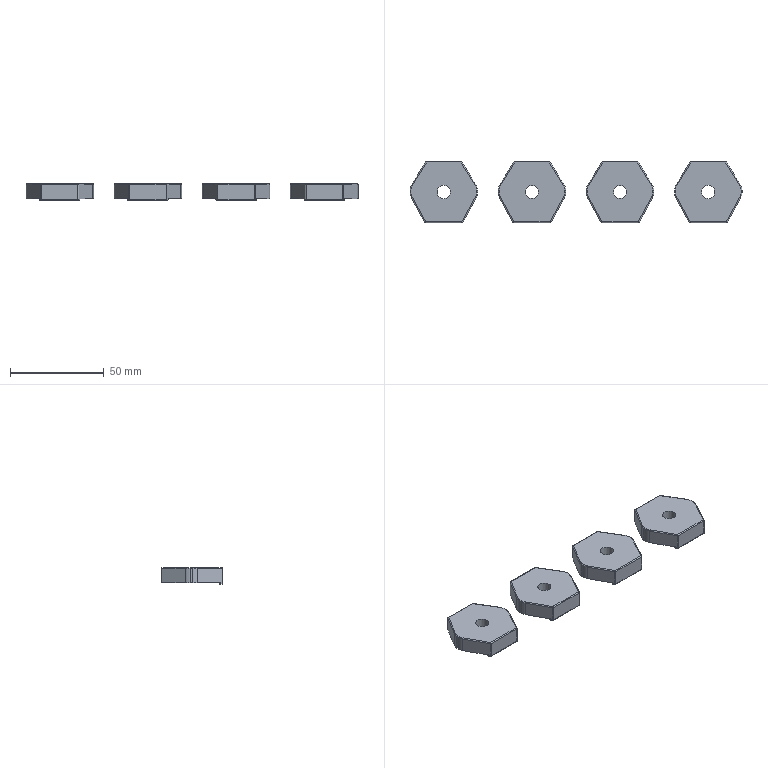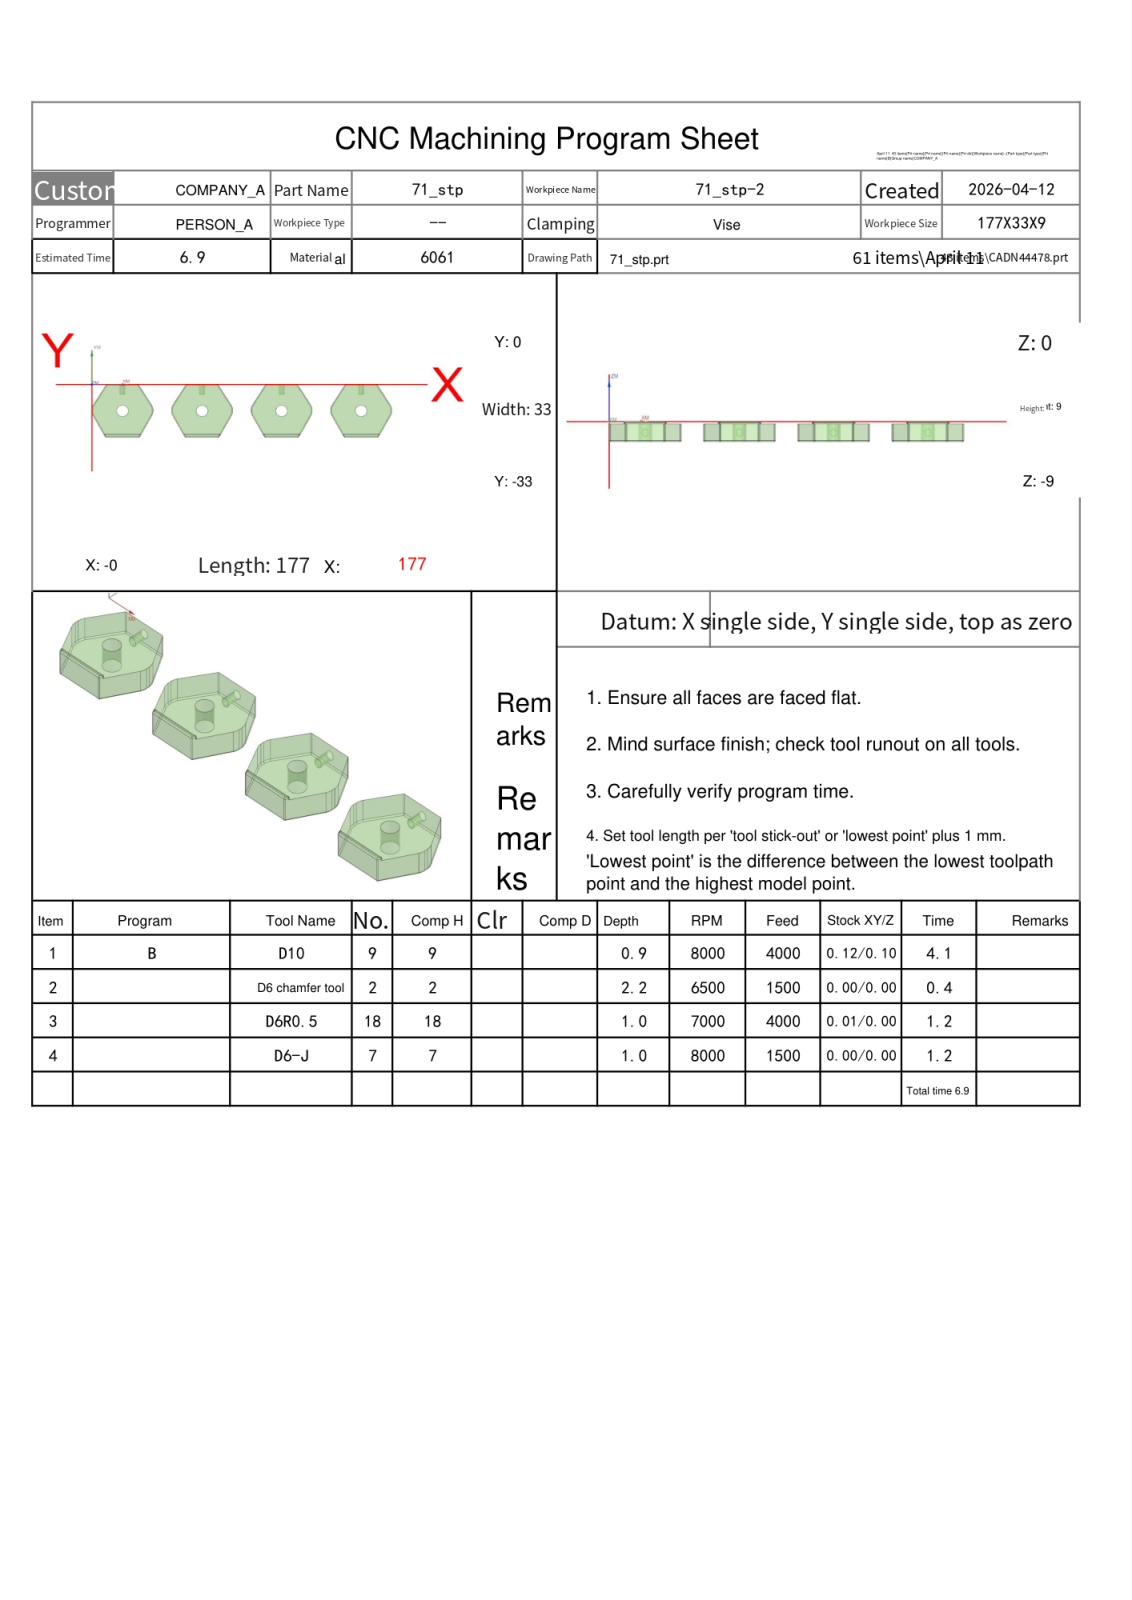NC program | NX | posted by the shop | part box 177 x 33 x 9 mm
Lines 2212 to 2352 of 12693:
N2 T02 M06
(D6 chamfer tool  D=6. R=0. H=02 ce=0.00 di=0.00)
G00 G90 G54 X5.559 Y-30.594 M03 S6500
G43 H02 Z50.
M08
Z1.8
G01 Z-2.2 F1500.
X-.275 Y-19.827
G02 X-1. Y-16.968 I5.275 J2.858
G01 Y-15.552
G02 X-.123 Y-12.428 I6. J0.0
G01 X7.627 Y.281
G02 X8.908 Y1. I1.281 J-.781
G01 X27.092
G02 X28.373 Y.281 I0.0 J-1.5
G01 X36.123 Y-12.428
G02 X37. Y-15.552 I-5.123 J-3.124
G01 Y-16.968
G02 X36.275 Y-19.827 I-6. J0.0
G01 X30.441 Y-30.594
Z1.8
G00 Z10.
X20.308 Y-16.904
Z-.749
G01 Z-2.2
G03 X20.482 Y-16.602 I-1.638 J1.147
G01 X20.508 Y-16.554
X20.5 Y-16.5
G03 X18. Y-14. I-2.5 J0.0
X15.5 Y-16.5 I0.0 J-2.5
X18. Y-19. I2.5 J0.0
X20.5 Y-16.5 I0.0 J2.5
G01 X20.508 Y-16.446
X20.482 Y-16.398
G03 X20.308 Y-16.096 I-1.813 J-.845
G01 Z-.749
G00 Z10.
X52.559 Y-30.594
Z1.8
G01 Z-2.2
X46.725 Y-19.827
G02 X46. Y-16.968 I5.275 J2.858
G01 Y-15.552
G02 X46.877 Y-12.428 I6. J0.0
G01 X54.627 Y.281
G02 X55.908 Y1. I1.281 J-.781
G01 X74.092
G02 X75.373 Y.281 I0.0 J-1.5
G01 X83.123 Y-12.428
G02 X84. Y-15.552 I-5.123 J-3.124
G01 Y-16.968
G02 X83.275 Y-19.827 I-6. J0.0
G01 X77.441 Y-30.594
Z1.8
G00 Z10.
X67.308 Y-16.904
Z-.749
G01 Z-2.2
G03 X67.482 Y-16.602 I-1.638 J1.147
G01 X67.508 Y-16.554
X67.5 Y-16.5
G03 X65. Y-14. I-2.5 J0.0
X62.5 Y-16.5 I0.0 J-2.5
X65. Y-19. I2.5 J0.0
X67.5 Y-16.5 I0.0 J2.5
G01 X67.508 Y-16.446
X67.482 Y-16.398
G03 X67.308 Y-16.096 I-1.813 J-.845
G01 Z-.749
G00 Z10.
X99.559 Y-30.594
Z1.8
G01 Z-2.2
X93.725 Y-19.827
G02 X93. Y-16.968 I5.275 J2.858
G01 Y-15.552
G02 X93.877 Y-12.428 I6. J0.0
G01 X101.627 Y.281
G02 X102.908 Y1. I1.281 J-.781
G01 X121.092
G02 X122.373 Y.281 I0.0 J-1.5
G01 X130.123 Y-12.428
G02 X131. Y-15.552 I-5.123 J-3.124
G01 Y-16.968
G02 X130.275 Y-19.827 I-6. J0.0
G01 X124.441 Y-30.594
Z1.8
G00 Z10.
X114.308 Y-16.904
Z-.749
G01 Z-2.2
G03 X114.482 Y-16.602 I-1.638 J1.147
G01 X114.508 Y-16.554
X114.5 Y-16.5
G03 X112. Y-14. I-2.5 J0.0
X109.5 Y-16.5 I0.0 J-2.5
X112. Y-19. I2.5 J0.0
X114.5 Y-16.5 I0.0 J2.5
G01 X114.508 Y-16.446
X114.482 Y-16.398
G03 X114.308 Y-16.096 I-1.813 J-.845
G01 Z-.749
G00 Z10.
X146.559 Y-30.594
Z1.8
G01 Z-2.2
X140.725 Y-19.827
G02 X140. Y-16.968 I5.275 J2.858
G01 Y-15.552
G02 X140.877 Y-12.428 I6. J0.0
G01 X148.627 Y.281
G02 X149.908 Y1. I1.281 J-.781
G01 X168.092
G02 X169.373 Y.281 I0.0 J-1.5
G01 X177.123 Y-12.428
G02 X178. Y-15.552 I-5.123 J-3.124
G01 Y-16.968
G02 X177.275 Y-19.827 I-6. J0.0
G01 X171.441 Y-30.594
Z1.8
G00 Z10.
X161.308 Y-16.904
Z-.749
G01 Z-2.2
G03 X161.482 Y-16.602 I-1.638 J1.147
G01 X161.508 Y-16.554
X161.5 Y-16.5
G03 X159. Y-14. I-2.5 J0.0
X156.5 Y-16.5 I0.0 J-2.5
X159. Y-19. I2.5 J0.0
X161.5 Y-16.5 I0.0 J2.5
G01 X161.508 Y-16.446
X161.482 Y-16.398
G03 X161.308 Y-16.096 I-1.813 J-.845
G01 Z-.749
G00 Z50.
G91 G28 Z0.0
M05
M09
G91 G28 Z0.0
M01